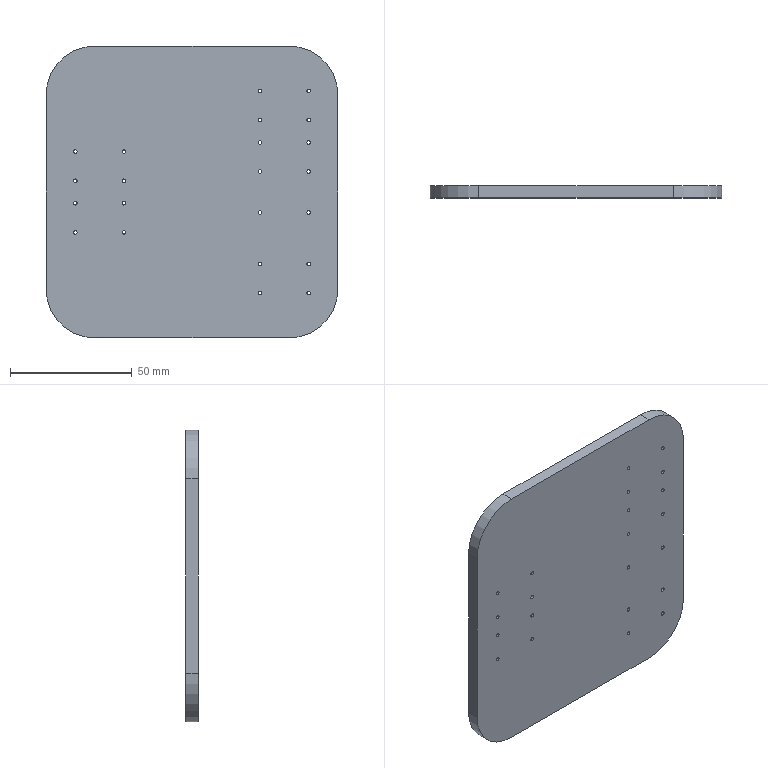Part | SolidWorks | features Extrusion 1, ICE 1 | 1 solid | 54 faces | box 120 x 5 x 120 mm | volume 70089 mm3 | cylinder 48 | plane 6 | commonest cylinder face diameters 1.5 x44 40 x4